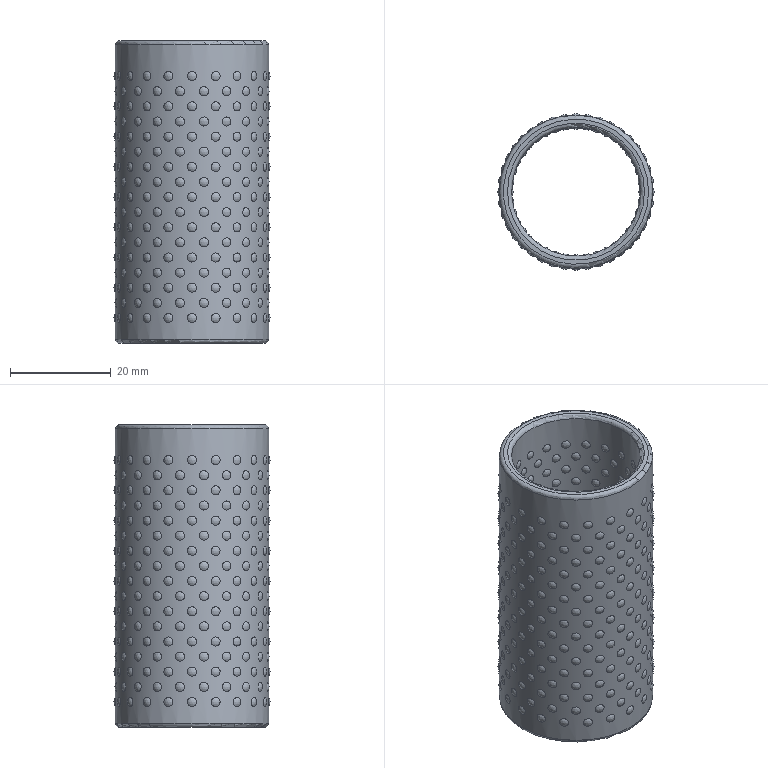Part | STEP file | 1 solid | 688 faces | box 31 x 31 x 60 mm | volume 12837 mm3 | sphere 680 | torus 4 | cylinder 2 | plane 2 | commonest cylinder face diameters 25.6 x1 30.4 x1